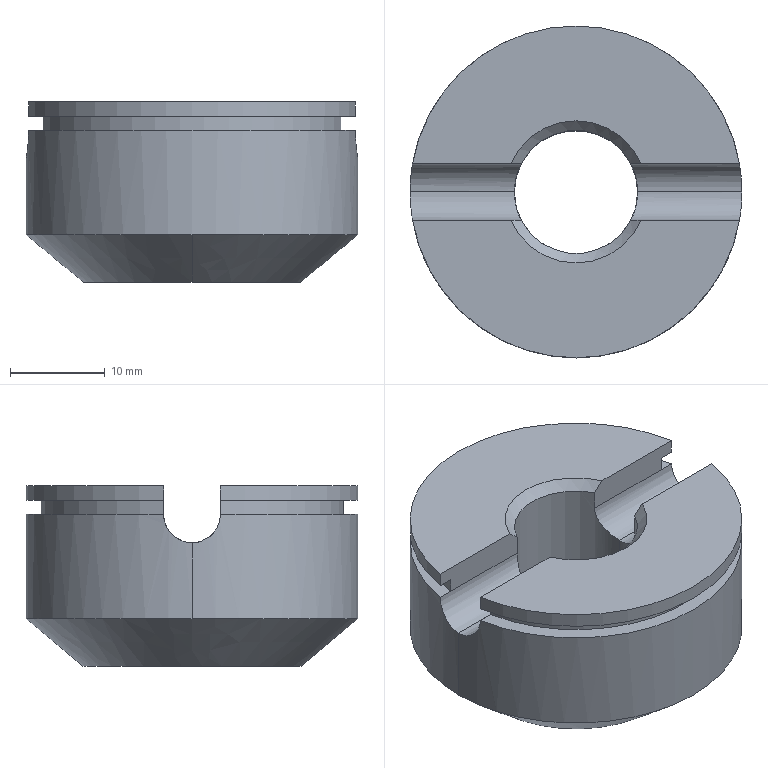Part | SolidWorks | features ICE 4, Blend 1, Chamfer 1, Extrusion 1 | 1 solid | 27 faces | box 35 x 35 x 19 mm | volume 13347 mm3 | cylinder 12 | plane 11 | spline 2 | cone 2 | commonest cylinder face diameters 6 x4 35 x4 13 x2 32 x2
STEP:
#1=CARTESIAN_POINT('',(0.,-17.5,0.));
#2=VERTEX_POINT('',#1);
#3=CARTESIAN_POINT('',(17.5,0.,0.));
#4=VERTEX_POINT('',#3);
#5=CARTESIAN_POINT('',(0.,0.,0.));
#6=DIRECTION('',(0.,0.,1.));
#7=DIRECTION('',(1.,0.,0.));
#8=AXIS2_PLACEMENT_3D('',#5,#6,#7);
#9=CIRCLE('',#8,17.5);
#10=EDGE_CURVE('',#2,#4,#9,.T.);
#11=ORIENTED_EDGE('',*,*,#10,.F.);
#12=CARTESIAN_POINT('',(0.,-11.5,-5.));
#13=VERTEX_POINT('',#12);
#14=CARTESIAN_POINT('',(0.,-17.5,0.));
#15=CARTESIAN_POINT('',(0.,-15.5,-1.667));
#16=CARTESIAN_POINT('',(0.,-13.5,-3.333));
#17=CARTESIAN_POINT('',(0.,-11.5,-5.));
#18=B_SPLINE_CURVE_WITH_KNOTS('',3,(#14,#15,#16,#17),.UNSPECIFIED.,.F.,.F.,(4,4),(0.,1.),.UNSPECIFIED.);
#19=EDGE_CURVE('',#2,#13,#18,.T.);
#20=ORIENTED_EDGE('',*,*,#19,.T.);
#21=CARTESIAN_POINT('',(0.,11.5,-5.));
#22=VERTEX_POINT('',#21);
#23=CARTESIAN_POINT('',(0.,0.,-5.));
#24=DIRECTION('',(0.,0.,-1.));
#25=DIRECTION('',(-1.,0.,0.));
#26=AXIS2_PLACEMENT_3D('',#23,#24,#25);
#27=CIRCLE('',#26,11.5);
#28=EDGE_CURVE('',#22,#13,#27,.T.);
#29=ORIENTED_EDGE('',*,*,#28,.F.);
#30=CARTESIAN_POINT('',(0.,17.5,0.));
#31=VERTEX_POINT('',#30);
#32=CARTESIAN_POINT('',(0.,17.5,0.));
#33=CARTESIAN_POINT('',(0.,15.5,-1.667));
#34=CARTESIAN_POINT('',(0.,13.5,-3.333));
#35=CARTESIAN_POINT('',(0.,11.5,-5.));
#36=B_SPLINE_CURVE_WITH_KNOTS('',3,(#32,#33,#34,#35),.UNSPECIFIED.,.F.,.F.,(4,4),(0.,1.),.UNSPECIFIED.);
#37=EDGE_CURVE('',#31,#22,#36,.T.);
#38=ORIENTED_EDGE('',*,*,#37,.F.);
#39=CARTESIAN_POINT('',(0.,0.,0.));
#40=DIRECTION('',(0.,0.,1.));
#41=DIRECTION('',(1.,0.,0.));
#42=AXIS2_PLACEMENT_3D('',#39,#40,#41);
#43=CIRCLE('',#42,17.5);
#44=EDGE_CURVE('',#4,#31,#43,.T.);
#45=ORIENTED_EDGE('',*,*,#44,.F.);
#46=EDGE_LOOP('',(#11,#20,#29,#38,#45));
#47=FACE_OUTER_BOUND('',#46,.T.);
#48=CARTESIAN_POINT('',(0.,17.5,0.));
#49=CARTESIAN_POINT('',(0.,15.5,-1.667));
#50=CARTESIAN_POINT('',(0.,13.5,-3.333));
#51=CARTESIAN_POINT('',(0.,11.5,-5.));
#52=CARTESIAN_POINT('',(0.4829,17.5,0.));
#53=CARTESIAN_POINT('',(0.4277,15.5,-1.667));
#54=CARTESIAN_POINT('',(0.3725,13.5,-3.333));
#55=CARTESIAN_POINT('',(0.3174,11.5,-5.));
#56=CARTESIAN_POINT('',(1.44,17.461,0.));
#57=CARTESIAN_POINT('',(1.275,15.465,-1.667));
#58=CARTESIAN_POINT('',(1.111,13.47,-3.333));
#59=CARTESIAN_POINT('',(0.9461,11.474,-5.));
#60=CARTESIAN_POINT('',(2.843,17.289,0.));
#61=CARTESIAN_POINT('',(2.518,15.313,-1.667));
#62=CARTESIAN_POINT('',(2.193,13.337,-3.333));
#63=CARTESIAN_POINT('',(1.868,11.361,-5.));
#64=CARTESIAN_POINT('',(4.21,17.008,0.));
#65=CARTESIAN_POINT('',(3.729,15.065,-1.667));
#66=CARTESIAN_POINT('',(3.248,13.121,-3.333));
#67=CARTESIAN_POINT('',(2.767,11.177,-5.));
#68=CARTESIAN_POINT('',(12.168,14.701,0.));
#69=CARTESIAN_POINT('',(10.777,13.021,-1.667));
#70=CARTESIAN_POINT('',(9.387,11.341,-3.333));
#71=CARTESIAN_POINT('',(7.996,9.661,-5.));
#72=CARTESIAN_POINT('',(17.5,7.727,0.));
#73=CARTESIAN_POINT('',(15.5,6.844,-1.667));
#74=CARTESIAN_POINT('',(13.5,5.961,-3.333));
#75=CARTESIAN_POINT('',(11.5,5.078,-5.));
#76=CARTESIAN_POINT('',(17.5,-9.659,0.));
#77=CARTESIAN_POINT('',(15.5,-8.555,-1.667));
#78=CARTESIAN_POINT('',(13.5,-7.451,-3.333));
#79=CARTESIAN_POINT('',(11.5,-6.347,-5.));
#80=CARTESIAN_POINT('',(9.659,-17.5,0.));
#81=CARTESIAN_POINT('',(8.555,-15.5,-1.667));
#82=CARTESIAN_POINT('',(7.451,-13.5,-3.333));
#83=CARTESIAN_POINT('',(6.347,-11.5,-5.));
#84=CARTESIAN_POINT('',(-9.659,-17.5,0.));
#85=CARTESIAN_POINT('',(-8.555,-15.5,-1.667));
#86=CARTESIAN_POINT('',(-7.451,-13.5,-3.333));
#87=CARTESIAN_POINT('',(-6.347,-11.5,-5.));
#88=CARTESIAN_POINT('',(-17.5,-9.659,0.));
#89=CARTESIAN_POINT('',(-15.5,-8.555,-1.667));
#90=CARTESIAN_POINT('',(-13.5,-7.451,-3.333));
#91=CARTESIAN_POINT('',(-11.5,-6.347,-5.));
#92=CARTESIAN_POINT('',(-17.5,7.727,0.));
#93=CARTESIAN_POINT('',(-15.5,6.844,-1.667));
#94=CARTESIAN_POINT('',(-13.5,5.961,-3.333));
#95=CARTESIAN_POINT('',(-11.5,5.078,-5.));
#96=CARTESIAN_POINT('',(-12.168,14.701,0.));
#97=CARTESIAN_POINT('',(-10.777,13.021,-1.667));
#98=CARTESIAN_POINT('',(-9.387,11.341,-3.333));
#99=CARTESIAN_POINT('',(-7.996,9.661,-5.));
#100=CARTESIAN_POINT('',(-4.21,17.008,0.));
#101=CARTESIAN_POINT('',(-3.729,15.065,-1.667));
#102=CARTESIAN_POINT('',(-3.248,13.121,-3.333));
#103=CARTESIAN_POINT('',(-2.767,11.177,-5.));
#104=CARTESIAN_POINT('',(-2.843,17.289,0.));
#105=CARTESIAN_POINT('',(-2.518,15.313,-1.667));
#106=CARTESIAN_POINT('',(-2.193,13.337,-3.333));
#107=CARTESIAN_POINT('',(-1.868,11.361,-5.));
#108=CARTESIAN_POINT('',(-1.44,17.461,0.));
#109=CARTESIAN_POINT('',(-1.275,15.465,-1.667));
#110=CARTESIAN_POINT('',(-1.111,13.47,-3.333));
#111=CARTESIAN_POINT('',(-0.9461,11.474,-5.));
#112=CARTESIAN_POINT('',(-0.4829,17.5,0.));
#113=CARTESIAN_POINT('',(-0.4277,15.5,-1.667));
#114=CARTESIAN_POINT('',(-0.3725,13.5,-3.333));
#115=CARTESIAN_POINT('',(-0.3174,11.5,-5.));
#116=CARTESIAN_POINT('',(0.,17.5,0.));
#117=CARTESIAN_POINT('',(0.,15.5,-1.667));
#118=CARTESIAN_POINT('',(0.,13.5,-3.333));
#119=CARTESIAN_POINT('',(0.,11.5,-5.));
#120=B_SPLINE_SURFACE_WITH_KNOTS('',3,3,((#48,#49,#50,#51),(#52,#53,#54,#55),(#56,#57,#58,#59),(#60,#61,#62,#63),(#64,#65,#66,#67),(#68,#69,#70,#71),(#72,#73,#74,#75),(#76,#77,#78,#79),(#80,#81,#82,#83),(#84,#85,#86,#87),(#88,#89,#90,#91),(#92,#93,#94,#95),(#96,#97,#98,#99),(#100,#101,#102,#103),(#104,#105,#106,#107),(#108,#109,#110,#111),(#112,#113,#114,#115),(#116,#117,#118,#119)),.UNSPECIFIED.,.T.,.F.,.F.,(4,1,1,1,1,2,2,2,1,1,1,1,4),(4,4),(0.,0.0125,0.025,0.0375,0.05,0.25,0.5,0.75,0.95,0.9625,0.975,0.9875,1.),(0.,1.),.UNSPECIFIED.);
#121=ADVANCED_FACE('',(#47),#120,.T.);
#122=CARTESIAN_POINT('',(-17.5,0.,8.));
#123=VERTEX_POINT('',#122);
#124=CARTESIAN_POINT('',(-17.241,3.,11.));
#125=VERTEX_POINT('',#124);
#126=CARTESIAN_POINT('',(-17.5,0.,8.));
#127=CARTESIAN_POINT('',(-17.5,0.1959,8.));
#128=CARTESIAN_POINT('',(-17.497,0.395,8.02));
#129=CARTESIAN_POINT('',(-17.484,0.7797,8.096));
#130=CARTESIAN_POINT('',(-17.474,0.9668,8.153));
#131=CARTESIAN_POINT('',(-17.45,1.33,8.304));
#132=CARTESIAN_POINT('',(-17.436,1.505,8.398));
#133=CARTESIAN_POINT('',(-17.405,1.83,8.614));
#134=CARTESIAN_POINT('',(-17.388,1.981,8.739));
#135=CARTESIAN_POINT('',(-17.354,2.261,9.018));
#136=CARTESIAN_POINT('',(-17.337,2.384,9.169));
#137=CARTESIAN_POINT('',(-17.306,2.601,9.493));
#138=CARTESIAN_POINT('',(-17.291,2.695,9.669));
#139=CARTESIAN_POINT('',(-17.267,2.846,10.031));
#140=CARTESIAN_POINT('',(-17.258,2.903,10.218));
#141=CARTESIAN_POINT('',(-17.244,2.98,10.603));
#142=CARTESIAN_POINT('',(-17.241,3.,10.802));
#143=CARTESIAN_POINT('',(-17.241,3.,11.));
#144=B_SPLINE_CURVE_WITH_KNOTS('',3,(#126,#127,#128,#129,#130,#131,#132,#133,#134,#135,#136,#137,#138,#139,#140,#141,#142,#143),.UNSPECIFIED.,.F.,.F.,(4,2,2,2,2,2,2,2,4),(0.004699,0.005286,0.005873,0.00646,0.007047,0.007634,0.008221,0.008807,0.009394),.UNSPECIFIED.);
#145=EDGE_CURVE('',#123,#125,#144,.T.);
#146=ORIENTED_EDGE('',*,*,#145,.F.);
#147=CARTESIAN_POINT('',(-6.5,0.,8.));
#148=VERTEX_POINT('',#147);
#149=CARTESIAN_POINT('',(-24.5,0.,8.));
#150=DIRECTION('',(1.,0.,0.));
#151=VECTOR('',#150,1000.);
#152=LINE('',#149,#151);
#153=EDGE_CURVE('',#123,#148,#152,.T.);
#154=ORIENTED_EDGE('',*,*,#153,.T.);
#155=CARTESIAN_POINT('',(-5.766,3.,11.));
#156=VERTEX_POINT('',#155);
#157=CARTESIAN_POINT('',(-5.766,3.,11.));
#158=CARTESIAN_POINT('',(-5.766,3.,10.799));
#159=CARTESIAN_POINT('',(-5.777,2.98,10.601));
#160=CARTESIAN_POINT('',(-5.816,2.902,10.214));
#161=CARTESIAN_POINT('',(-5.846,2.843,10.022));
#162=CARTESIAN_POINT('',(-5.917,2.691,9.66));
#163=CARTESIAN_POINT('',(-5.959,2.599,9.489));
#164=CARTESIAN_POINT('',(-6.049,2.382,9.165));
#165=CARTESIAN_POINT('',(-6.097,2.257,9.015));
#166=CARTESIAN_POINT('',(-6.191,1.985,8.742));
#167=CARTESIAN_POINT('',(-6.238,1.834,8.618));
#168=CARTESIAN_POINT('',(-6.325,1.509,8.4));
#169=CARTESIAN_POINT('',(-6.363,1.338,8.308));
#170=CARTESIAN_POINT('',(-6.429,0.9774,8.157));
#171=CARTESIAN_POINT('',(-6.455,0.7852,8.098));
#172=CARTESIAN_POINT('',(-6.491,0.3961,8.02));
#173=CARTESIAN_POINT('',(-6.5,0.1993,8.));
#174=CARTESIAN_POINT('',(-6.5,0.,8.));
#175=B_SPLINE_CURVE_WITH_KNOTS('',3,(#157,#158,#159,#160,#161,#162,#163,#164,#165,#166,#167,#168,#169,#170,#171,#172,#173,#174),.UNSPECIFIED.,.F.,.F.,(4,2,2,2,2,2,2,2,4),(0.,0.0005949,0.00119,0.001785,0.00238,0.002975,0.00357,0.004165,0.004759),.UNSPECIFIED.);
#176=EDGE_CURVE('',#156,#148,#175,.T.);
#177=ORIENTED_EDGE('',*,*,#176,.F.);
#178=CARTESIAN_POINT('',(-15.716,3.,11.));
#179=VERTEX_POINT('',#178);
#180=CARTESIAN_POINT('',(-24.5,3.,11.));
#181=DIRECTION('',(1.,0.,0.));
#182=VECTOR('',#181,1000.);
#183=LINE('',#180,#182);
#184=EDGE_CURVE('',#179,#156,#183,.T.);
#185=ORIENTED_EDGE('',*,*,#184,.F.);
#186=CARTESIAN_POINT('',(-24.5,3.,11.));
#187=DIRECTION('',(1.,0.,0.));
#188=VECTOR('',#187,1000.);
#189=LINE('',#186,#188);
#190=EDGE_CURVE('',#125,#179,#189,.T.);
#191=ORIENTED_EDGE('',*,*,#190,.F.);
#192=EDGE_LOOP('',(#146,#154,#177,#185,#191));
#193=FACE_OUTER_BOUND('',#192,.T.);
#194=CARTESIAN_POINT('',(-24.5,0.,11.));
#195=DIRECTION('',(1.,0.,0.));
#196=DIRECTION('',(0.,0.,-1.));
#197=AXIS2_PLACEMENT_3D('',#194,#195,#196);
#198=CYLINDRICAL_SURFACE('',#197,3.);
#199=ADVANCED_FACE('',(#193),#198,.F.);
#200=CARTESIAN_POINT('',(6.5,0.,8.));
#201=VERTEX_POINT('',#200);
#202=CARTESIAN_POINT('',(5.766,3.,11.));
#203=VERTEX_POINT('',#202);
#204=CARTESIAN_POINT('',(6.5,0.,8.));
#205=CARTESIAN_POINT('',(6.5,0.1989,8.));
#206=CARTESIAN_POINT('',(6.491,0.4002,8.02));
#207=CARTESIAN_POINT('',(6.455,0.7874,8.098));
#208=CARTESIAN_POINT('',(6.429,0.9772,8.157));
#209=CARTESIAN_POINT('',(6.363,1.342,8.309));
#210=CARTESIAN_POINT('',(6.324,1.513,8.402));
#211=CARTESIAN_POINT('',(6.238,1.835,8.619));
#212=CARTESIAN_POINT('',(6.191,1.987,8.744));
#213=CARTESIAN_POINT('',(6.096,2.259,9.017));
#214=CARTESIAN_POINT('',(6.049,2.382,9.166));
#215=CARTESIAN_POINT('',(5.959,2.599,9.489));
#216=CARTESIAN_POINT('',(5.917,2.692,9.662));
#217=CARTESIAN_POINT('',(5.811,2.917,10.2));
#218=CARTESIAN_POINT('',(5.766,3.,10.598));
#219=CARTESIAN_POINT('',(5.766,3.,11.));
#220=B_SPLINE_CURVE_WITH_KNOTS('',3,(#204,#205,#206,#207,#208,#209,#210,#211,#212,#213,#214,#215,#216,#217,#218,#219),.UNSPECIFIED.,.F.,.F.,(4,2,2,2,2,2,2,4),(0.004759,0.005353,0.005947,0.006541,0.007135,0.007729,0.008323,0.00951),.UNSPECIFIED.);
#221=EDGE_CURVE('',#201,#203,#220,.T.);
#222=ORIENTED_EDGE('',*,*,#221,.F.);
#223=CARTESIAN_POINT('',(17.5,0.,8.));
#224=VERTEX_POINT('',#223);
#225=CARTESIAN_POINT('',(-24.5,0.,8.));
#226=DIRECTION('',(1.,0.,0.));
#227=VECTOR('',#226,1000.);
#228=LINE('',#225,#227);
#229=EDGE_CURVE('',#201,#224,#228,.T.);
#230=ORIENTED_EDGE('',*,*,#229,.T.);
#231=CARTESIAN_POINT('',(17.241,3.,11.));
#232=VERTEX_POINT('',#231);
#233=CARTESIAN_POINT('',(17.241,3.,11.));
#234=CARTESIAN_POINT('',(17.241,3.,10.801));
#235=CARTESIAN_POINT('',(17.244,2.98,10.606));
#236=CARTESIAN_POINT('',(17.257,2.904,10.222));
#237=CARTESIAN_POINT('',(17.267,2.846,10.031));
#238=CARTESIAN_POINT('',(17.291,2.695,9.668));
#239=CARTESIAN_POINT('',(17.306,2.603,9.496));
#240=CARTESIAN_POINT('',(17.337,2.385,9.17));
#241=CARTESIAN_POINT('',(17.354,2.259,9.016));
#242=CARTESIAN_POINT('',(17.388,1.982,8.74));
#243=CARTESIAN_POINT('',(17.405,1.831,8.616));
#244=CARTESIAN_POINT('',(17.436,1.503,8.396));
#245=CARTESIAN_POINT('',(17.45,1.329,8.303));
#246=CARTESIAN_POINT('',(17.474,0.9682,8.154));
#247=CARTESIAN_POINT('',(17.484,0.7787,8.096));
#248=CARTESIAN_POINT('',(17.497,0.3911,8.019));
#249=CARTESIAN_POINT('',(17.5,0.1961,8.));
#250=CARTESIAN_POINT('',(17.5,0.,8.));
#251=B_SPLINE_CURVE_WITH_KNOTS('',3,(#233,#234,#235,#236,#237,#238,#239,#240,#241,#242,#243,#244,#245,#246,#247,#248,#249,#250),.UNSPECIFIED.,.F.,.F.,(4,2,2,2,2,2,2,2,4),(0.,0.0005874,0.001175,0.001762,0.00235,0.002937,0.003525,0.004112,0.004699),.UNSPECIFIED.);
#252=EDGE_CURVE('',#232,#224,#251,.T.);
#253=ORIENTED_EDGE('',*,*,#252,.F.);
#254=CARTESIAN_POINT('',(15.716,3.,11.));
#255=VERTEX_POINT('',#254);
#256=CARTESIAN_POINT('',(-24.5,3.,11.));
#257=DIRECTION('',(1.,0.,0.));
#258=VECTOR('',#257,1000.);
#259=LINE('',#256,#258);
#260=EDGE_CURVE('',#255,#232,#259,.T.);
#261=ORIENTED_EDGE('',*,*,#260,.F.);
#262=CARTESIAN_POINT('',(-24.5,3.,11.));
#263=DIRECTION('',(1.,0.,0.));
#264=VECTOR('',#263,1000.);
#265=LINE('',#262,#264);
#266=EDGE_CURVE('',#203,#255,#265,.T.);
#267=ORIENTED_EDGE('',*,*,#266,.F.);
#268=EDGE_LOOP('',(#222,#230,#253,#261,#267));
#269=FACE_OUTER_BOUND('',#268,.T.);
#270=CARTESIAN_POINT('',(-24.5,0.,11.));
#271=DIRECTION('',(1.,0.,0.));
#272=DIRECTION('',(0.,0.,-1.));
#273=AXIS2_PLACEMENT_3D('',#270,#271,#272);
#274=CYLINDRICAL_SURFACE('',#273,3.);
#275=ADVANCED_FACE('',(#269),#274,.F.);
#276=CARTESIAN_POINT('',(6.5,0.,-5.));
#277=VERTEX_POINT('',#276);
#278=CARTESIAN_POINT('',(-6.5,0.,-5.));
#279=VERTEX_POINT('',#278);
#280=CARTESIAN_POINT('',(0.,0.,-5.));
#281=DIRECTION('',(0.,0.,-1.));
#282=DIRECTION('',(-1.,0.,0.));
#283=AXIS2_PLACEMENT_3D('',#280,#281,#282);
#284=CIRCLE('',#283,6.5);
#285=EDGE_CURVE('',#277,#279,#284,.T.);
#286=ORIENTED_EDGE('',*,*,#285,.T.);
#287=CARTESIAN_POINT('',(-6.5,0.,-5.));
#288=DIRECTION('',(0.,0.,1.));
#289=VECTOR('',#288,1000.);
#290=LINE('',#287,#289);
#291=EDGE_CURVE('',#279,#148,#290,.T.);
#292=ORIENTED_EDGE('',*,*,#291,.T.);
#293=CARTESIAN_POINT('',(-5.766,-3.,11.));
#294=VERTEX_POINT('',#293);
#295=CARTESIAN_POINT('',(-6.5,0.,8.));
#296=CARTESIAN_POINT('',(-6.5,-0.1989,8.));
#297=CARTESIAN_POINT('',(-6.491,-0.4002,8.02));
#298=CARTESIAN_POINT('',(-6.455,-0.7874,8.098));
#299=CARTESIAN_POINT('',(-6.429,-0.9772,8.157));
#300=CARTESIAN_POINT('',(-6.363,-1.342,8.309));
#301=CARTESIAN_POINT('',(-6.324,-1.513,8.402));
#302=CARTESIAN_POINT('',(-6.238,-1.835,8.619));
#303=CARTESIAN_POINT('',(-6.191,-1.987,8.744));
#304=CARTESIAN_POINT('',(-6.096,-2.259,9.017));
#305=CARTESIAN_POINT('',(-6.049,-2.382,9.166));
#306=CARTESIAN_POINT('',(-5.959,-2.599,9.489));
#307=CARTESIAN_POINT('',(-5.917,-2.692,9.662));
#308=CARTESIAN_POINT('',(-5.811,-2.917,10.2));
#309=CARTESIAN_POINT('',(-5.766,-3.,10.598));
#310=CARTESIAN_POINT('',(-5.766,-3.,11.));
#311=B_SPLINE_CURVE_WITH_KNOTS('',3,(#295,#296,#297,#298,#299,#300,#301,#302,#303,#304,#305,#306,#307,#308,#309,#310),.UNSPECIFIED.,.F.,.F.,(4,2,2,2,2,2,2,4),(0.004759,0.005353,0.005947,0.006541,0.007135,0.007729,0.008323,0.00951),.UNSPECIFIED.);
#312=EDGE_CURVE('',#148,#294,#311,.T.);
#313=ORIENTED_EDGE('',*,*,#312,.T.);
#314=CARTESIAN_POINT('',(-5.766,-3.,13.));
#315=VERTEX_POINT('',#314);
#316=CARTESIAN_POINT('',(-5.766,-3.,-5.));
#317=DIRECTION('',(0.,0.,1.));
#318=VECTOR('',#317,1000.);
#319=LINE('',#316,#318);
#320=EDGE_CURVE('',#294,#315,#319,.T.);
#321=ORIENTED_EDGE('',*,*,#320,.T.);
#322=CARTESIAN_POINT('',(5.766,-3.,13.));
#323=VERTEX_POINT('',#322);
#324=CARTESIAN_POINT('',(0.,0.,13.));
#325=DIRECTION('',(0.,0.,1.));
#326=DIRECTION('',(1.,0.,0.));
#327=AXIS2_PLACEMENT_3D('',#324,#325,#326);
#328=CIRCLE('',#327,6.5);
#329=EDGE_CURVE('',#315,#323,#328,.T.);
#330=ORIENTED_EDGE('',*,*,#329,.T.);
#331=CARTESIAN_POINT('',(5.766,-3.,11.));
#332=VERTEX_POINT('',#331);
#333=CARTESIAN_POINT('',(5.766,-3.,-5.));
#334=DIRECTION('',(0.,0.,-1.));
#335=VECTOR('',#334,1000.);
#336=LINE('',#333,#335);
#337=EDGE_CURVE('',#323,#332,#336,.T.);
#338=ORIENTED_EDGE('',*,*,#337,.T.);
#339=CARTESIAN_POINT('',(5.766,-3.,11.));
#340=CARTESIAN_POINT('',(5.766,-3.,10.799));
#341=CARTESIAN_POINT('',(5.777,-2.98,10.601));
#342=CARTESIAN_POINT('',(5.816,-2.902,10.214));
#343=CARTESIAN_POINT('',(5.846,-2.843,10.022));
#344=CARTESIAN_POINT('',(5.917,-2.691,9.66));
#345=CARTESIAN_POINT('',(5.959,-2.599,9.489));
#346=CARTESIAN_POINT('',(6.049,-2.382,9.165));
#347=CARTESIAN_POINT('',(6.097,-2.257,9.015));
#348=CARTESIAN_POINT('',(6.191,-1.985,8.742));
#349=CARTESIAN_POINT('',(6.238,-1.834,8.618));
#350=CARTESIAN_POINT('',(6.325,-1.509,8.4));
#351=CARTESIAN_POINT('',(6.363,-1.338,8.308));
#352=CARTESIAN_POINT('',(6.429,-0.9774,8.157));
#353=CARTESIAN_POINT('',(6.455,-0.7852,8.098));
#354=CARTESIAN_POINT('',(6.491,-0.3961,8.02));
#355=CARTESIAN_POINT('',(6.5,-0.1993,8.));
#356=CARTESIAN_POINT('',(6.5,0.,8.));
#357=B_SPLINE_CURVE_WITH_KNOTS('',3,(#339,#340,#341,#342,#343,#344,#345,#346,#347,#348,#349,#350,#351,#352,#353,#354,#355,#356),.UNSPECIFIED.,.F.,.F.,(4,2,2,2,2,2,2,2,4),(0.,0.0005949,0.00119,0.001785,0.00238,0.002975,0.00357,0.004165,0.004759),.UNSPECIFIED.);
#358=EDGE_CURVE('',#332,#201,#357,.T.);
#359=ORIENTED_EDGE('',*,*,#358,.T.);
#360=CARTESIAN_POINT('',(6.5,0.,-5.));
#361=DIRECTION('',(0.,0.,1.));
#362=VECTOR('',#361,1000.);
#363=LINE('',#360,#362);
#364=EDGE_CURVE('',#277,#201,#363,.T.);
#365=ORIENTED_EDGE('',*,*,#364,.F.);
#366=EDGE_LOOP('',(#286,#292,#313,#321,#330,#338,#359,#365));
#367=FACE_OUTER_BOUND('',#366,.T.);
#368=CARTESIAN_POINT('',(0.,0.,-5.));
#369=DIRECTION('',(0.,0.,1.));
#370=DIRECTION('',(1.,0.,0.));
#371=AXIS2_PLACEMENT_3D('',#368,#369,#370);
#372=CYLINDRICAL_SURFACE('',#371,6.5);
#373=ADVANCED_FACE('',(#367),#372,.F.);
#374=ORIENTED_EDGE('',*,*,#252,.T.);
#375=CARTESIAN_POINT('',(17.5,0.,14.));
#376=DIRECTION('',(0.,0.,-1.));
#377=VECTOR('',#376,1000.);
#378=LINE('',#375,#377);
#379=EDGE_CURVE('',#224,#4,#378,.T.);
#380=ORIENTED_EDGE('',*,*,#379,.T.);
#381=ORIENTED_EDGE('',*,*,#44,.T.);
#382=CARTESIAN_POINT('',(-17.5,0.,0.));
#383=VERTEX_POINT('',#382);
#384=CARTESIAN_POINT('',(0.,0.,0.));
#385=DIRECTION('',(0.,0.,1.));
#386=DIRECTION('',(1.,0.,0.));
#387=AXIS2_PLACEMENT_3D('',#384,#385,#386);
#388=CIRCLE('',#387,17.5);
#389=EDGE_CURVE('',#31,#383,#388,.T.);
#390=ORIENTED_EDGE('',*,*,#389,.T.);
#391=CARTESIAN_POINT('',(-17.5,0.,14.));
#392=DIRECTION('',(0.,0.,-1.));
#393=VECTOR('',#392,1000.);
#394=LINE('',#391,#393);
#395=EDGE_CURVE('',#123,#383,#394,.T.);
#396=ORIENTED_EDGE('',*,*,#395,.F.);
#397=ORIENTED_EDGE('',*,*,#145,.T.);
#398=CARTESIAN_POINT('',(0.,0.,11.));
#399=DIRECTION('',(0.,0.,1.));
#400=DIRECTION('',(1.,0.,0.));
#401=AXIS2_PLACEMENT_3D('',#398,#399,#400);
#402=CIRCLE('',#401,17.5);
#403=EDGE_CURVE('',#232,#125,#402,.T.);
#404=ORIENTED_EDGE('',*,*,#403,.F.);
#405=EDGE_LOOP('',(#374,#380,#381,#390,#396,#397,#404));
#406=FACE_OUTER_BOUND('',#405,.T.);
#407=CARTESIAN_POINT('',(0.,0.,14.));
#408=DIRECTION('',(0.,0.,-1.));
#409=DIRECTION('',(-1.,0.,0.));
#410=AXIS2_PLACEMENT_3D('',#407,#408,#409);
#411=CYLINDRICAL_SURFACE('',#410,17.5);
#412=ADVANCED_FACE('',(#406),#411,.T.);
#413=ORIENTED_EDGE('',*,*,#379,.F.);
#414=CARTESIAN_POINT('',(17.241,-3.,11.));
#415=VERTEX_POINT('',#414);
#416=CARTESIAN_POINT('',(17.5,0.,8.));
#417=CARTESIAN_POINT('',(17.5,-0.1959,8.));
#418=CARTESIAN_POINT('',(17.497,-0.395,8.02));
#419=CARTESIAN_POINT('',(17.484,-0.7797,8.096));
#420=CARTESIAN_POINT('',(17.474,-0.9668,8.153));
#421=CARTESIAN_POINT('',(17.45,-1.33,8.304));
#422=CARTESIAN_POINT('',(17.436,-1.505,8.398));
#423=CARTESIAN_POINT('',(17.405,-1.83,8.614));
#424=CARTESIAN_POINT('',(17.388,-1.981,8.739));
#425=CARTESIAN_POINT('',(17.354,-2.261,9.018));
#426=CARTESIAN_POINT('',(17.337,-2.384,9.169));
#427=CARTESIAN_POINT('',(17.306,-2.601,9.493));
#428=CARTESIAN_POINT('',(17.291,-2.695,9.669));
#429=CARTESIAN_POINT('',(17.267,-2.846,10.031));
#430=CARTESIAN_POINT('',(17.258,-2.903,10.218));
#431=CARTESIAN_POINT('',(17.244,-2.98,10.603));
#432=CARTESIAN_POINT('',(17.241,-3.,10.802));
#433=CARTESIAN_POINT('',(17.241,-3.,11.));
#434=B_SPLINE_CURVE_WITH_KNOTS('',3,(#416,#417,#418,#419,#420,#421,#422,#423,#424,#425,#426,#427,#428,#429,#430,#431,#432,#433),.UNSPECIFIED.,.F.,.F.,(4,2,2,2,2,2,2,2,4),(0.004699,0.005286,0.005873,0.00646,0.007047,0.007634,0.008221,0.008807,0.009394),.UNSPECIFIED.);
#435=EDGE_CURVE('',#224,#415,#434,.T.);
#436=ORIENTED_EDGE('',*,*,#435,.T.);
#437=CARTESIAN_POINT('',(-17.241,-3.,11.));
#438=VERTEX_POINT('',#437);
#439=CARTESIAN_POINT('',(0.,0.,11.));
#440=DIRECTION('',(0.,0.,1.));
#441=DIRECTION('',(1.,0.,0.));
#442=AXIS2_PLACEMENT_3D('',#439,#440,#441);
#443=CIRCLE('',#442,17.5);
#444=EDGE_CURVE('',#438,#415,#443,.T.);
#445=ORIENTED_EDGE('',*,*,#444,.F.);
#446=CARTESIAN_POINT('',(-17.241,-3.,11.));
#447=CARTESIAN_POINT('',(-17.241,-3.,10.801));
#448=CARTESIAN_POINT('',(-17.244,-2.98,10.606));
#449=CARTESIAN_POINT('',(-17.257,-2.904,10.222));
#450=CARTESIAN_POINT('',(-17.267,-2.846,10.031));
#451=CARTESIAN_POINT('',(-17.291,-2.695,9.668));
#452=CARTESIAN_POINT('',(-17.306,-2.603,9.496));
#453=CARTESIAN_POINT('',(-17.337,-2.385,9.17));
#454=CARTESIAN_POINT('',(-17.354,-2.259,9.016));
#455=CARTESIAN_POINT('',(-17.388,-1.982,8.74));
#456=CARTESIAN_POINT('',(-17.405,-1.831,8.616));
#457=CARTESIAN_POINT('',(-17.436,-1.503,8.396));
#458=CARTESIAN_POINT('',(-17.45,-1.329,8.303));
#459=CARTESIAN_POINT('',(-17.474,-0.9682,8.154));
#460=CARTESIAN_POINT('',(-17.484,-0.7787,8.096));
#461=CARTESIAN_POINT('',(-17.497,-0.3911,8.019));
#462=CARTESIAN_POINT('',(-17.5,-0.1961,8.));
#463=CARTESIAN_POINT('',(-17.5,0.,8.));
#464=B_SPLINE_CURVE_WITH_KNOTS('',3,(#446,#447,#448,#449,#450,#451,#452,#453,#454,#455,#456,#457,#458,#459,#460,#461,#462,#463),.UNSPECIFIED.,.F.,.F.,(4,2,2,2,2,2,2,2,4),(0.,0.0005874,0.001175,0.001762,0.00235,0.002937,0.003525,0.004112,0.004699),.UNSPECIFIED.);
#465=EDGE_CURVE('',#438,#123,#464,.T.);
#466=ORIENTED_EDGE('',*,*,#465,.T.);
#467=ORIENTED_EDGE('',*,*,#395,.T.);
#468=CARTESIAN_POINT('',(0.,0.,0.));
#469=DIRECTION('',(0.,0.,1.));
#470=DIRECTION('',(1.,0.,0.));
#471=AXIS2_PLACEMENT_3D('',#468,#469,#470);
#472=CIRCLE('',#471,17.5);
#473=EDGE_CURVE('',#383,#2,#472,.T.);
#474=ORIENTED_EDGE('',*,*,#473,.T.);
#475=ORIENTED_EDGE('',*,*,#10,.T.);
#476=EDGE_LOOP('',(#413,#436,#445,#466,#467,#474,#475));
#477=FACE_OUTER_BOUND('',#476,.T.);
#478=CARTESIAN_POINT('',(0.,0.,14.));
#479=DIRECTION('',(0.,0.,-1.));
#480=DIRECTION('',(-1.,0.,0.));
#481=AXIS2_PLACEMENT_3D('',#478,#479,#480);
#482=CYLINDRICAL_SURFACE('',#481,17.5);
#483=ADVANCED_FACE('',(#477),#482,.T.);
#484=CARTESIAN_POINT('',(17.241,3.,14.));
#485=VERTEX_POINT('',#484);
#486=CARTESIAN_POINT('',(17.241,3.,12.5));
#487=VERTEX_POINT('',#486);
#488=CARTESIAN_POINT('',(17.241,3.,14.));
#489=DIRECTION('',(0.,0.,-1.));
#490=VECTOR('',#489,1000.);
#491=LINE('',#488,#490);
#492=EDGE_CURVE('',#485,#487,#491,.T.);
#493=ORIENTED_EDGE('',*,*,#492,.T.);
#494=CARTESIAN_POINT('',(-17.241,3.,12.5));
#495=VERTEX_POINT('',#494);
#496=CARTESIAN_POINT('',(0.,0.,12.5));
#497=DIRECTION('',(0.,0.,1.));
#498=DIRECTION('',(1.,0.,0.));
#499=AXIS2_PLACEMENT_3D('',#496,#497,#498);
#500=CIRCLE('',#499,17.5);
#501=EDGE_CURVE('',#487,#495,#500,.T.);
#502=ORIENTED_EDGE('',*,*,#501,.T.);
#503=CARTESIAN_POINT('',(-17.241,3.,14.));
#504=VERTEX_POINT('',#503);
#505=CARTESIAN_POINT('',(-17.241,3.,14.));
#506=DIRECTION('',(0.,0.,1.));
#507=VECTOR('',#506,1000.);
#508=LINE('',#505,#507);
#509=EDGE_CURVE('',#495,#504,#508,.T.);
#510=ORIENTED_EDGE('',*,*,#509,.T.);
#511=CARTESIAN_POINT('',(0.,0.,14.));
#512=DIRECTION('',(0.,0.,1.));
#513=DIRECTION('',(1.,0.,0.));
#514=AXIS2_PLACEMENT_3D('',#511,#512,#513);
#515=CIRCLE('',#514,17.5);
#516=EDGE_CURVE('',#485,#504,#515,.T.);
#517=ORIENTED_EDGE('',*,*,#516,.F.);
#518=EDGE_LOOP('',(#493,#502,#510,#517));
#519=FACE_OUTER_BOUND('',#518,.T.);
#520=CARTESIAN_POINT('',(0.,0.,14.));
#521=DIRECTION('',(0.,0.,-1.));
#522=DIRECTION('',(-1.,0.,0.));
#523=AXIS2_PLACEMENT_3D('',#520,#521,#522);
#524=CYLINDRICAL_SURFACE('',#523,17.5);
#525=ADVANCED_FACE('',(#519),#524,.T.);
#526=CARTESIAN_POINT('',(6.874,-3.,14.));
#527=VERTEX_POINT('',#526);
#528=CARTESIAN_POINT('',(17.241,-3.,14.));
#529=VERTEX_POINT('',#528);
#530=CARTESIAN_POINT('',(-24.5,-3.,14.));
#531=DIRECTION('',(1.,0.,0.));
#532=VECTOR('',#531,1000.);
#533=LINE('',#530,#532);
#534=EDGE_CURVE('',#527,#529,#533,.T.);
#535=ORIENTED_EDGE('',*,*,#534,.F.);
#536=CARTESIAN_POINT('',(-6.874,-3.,14.));
#537=VERTEX_POINT('',#536);
#538=CARTESIAN_POINT('',(0.,0.,14.));
#539=DIRECTION('',(0.,0.,-1.));
#540=DIRECTION('',(1.,0.,0.));
#541=AXIS2_PLACEMENT_3D('',#538,#539,#540);
#542=CIRCLE('',#541,7.5);
#543=EDGE_CURVE('',#527,#537,#542,.T.);
#544=ORIENTED_EDGE('',*,*,#543,.T.);
#545=CARTESIAN_POINT('',(-17.241,-3.,14.));
#546=VERTEX_POINT('',#545);
#547=CARTESIAN_POINT('',(-24.5,-3.,14.));
#548=DIRECTION('',(1.,0.,0.));
#549=VECTOR('',#548,1000.);
#550=LINE('',#547,#549);
#551=EDGE_CURVE('',#546,#537,#550,.T.);
#552=ORIENTED_EDGE('',*,*,#551,.F.);
#553=CARTESIAN_POINT('',(0.,0.,14.));
#554=DIRECTION('',(0.,0.,1.));
#555=DIRECTION('',(1.,0.,0.));
#556=AXIS2_PLACEMENT_3D('',#553,#554,#555);
#557=CIRCLE('',#556,17.5);
#558=EDGE_CURVE('',#546,#529,#557,.T.);
#559=ORIENTED_EDGE('',*,*,#558,.T.);
#560=EDGE_LOOP('',(#535,#544,#552,#559));
#561=FACE_OUTER_BOUND('',#560,.T.);
#562=CARTESIAN_POINT('',(0.,0.,14.));
#563=DIRECTION('',(0.,0.,1.));
#564=DIRECTION('',(1.,0.,0.));
#565=AXIS2_PLACEMENT_3D('',#562,#563,#564);
#566=PLANE('',#565);
#567=ADVANCED_FACE('',(#561),#566,.T.);
#568=CARTESIAN_POINT('',(-17.241,-3.,12.5));
#569=VERTEX_POINT('',#568);
#570=CARTESIAN_POINT('',(-17.241,-3.,14.));
#571=DIRECTION('',(0.,0.,-1.));
#572=VECTOR('',#571,1000.);
#573=LINE('',#570,#572);
#574=EDGE_CURVE('',#546,#569,#573,.T.);
#575=ORIENTED_EDGE('',*,*,#574,.T.);
#576=CARTESIAN_POINT('',(17.241,-3.,12.5));
#577=VERTEX_POINT('',#576);
#578=CARTESIAN_POINT('',(0.,0.,12.5));
#579=DIRECTION('',(0.,0.,1.));
#580=DIRECTION('',(1.,0.,0.));
#581=AXIS2_PLACEMENT_3D('',#578,#579,#580);
#582=CIRCLE('',#581,17.5);
#583=EDGE_CURVE('',#569,#577,#582,.T.);
#584=ORIENTED_EDGE('',*,*,#583,.T.);
#585=CARTESIAN_POINT('',(17.241,-3.,14.));
#586=DIRECTION('',(0.,0.,1.));
#587=VECTOR('',#586,1000.);
#588=LINE('',#585,#587);
#589=EDGE_CURVE('',#577,#529,#588,.T.);
#590=ORIENTED_EDGE('',*,*,#589,.T.);
#591=ORIENTED_EDGE('',*,*,#558,.F.);
#592=EDGE_LOOP('',(#575,#584,#590,#591));
#593=FACE_OUTER_BOUND('',#592,.T.);
#594=CARTESIAN_POINT('',(0.,0.,14.));
#595=DIRECTION('',(0.,0.,-1.));
#596=DIRECTION('',(-1.,0.,0.));
#597=AXIS2_PLACEMENT_3D('',#594,#595,#596);
#598=CYLINDRICAL_SURFACE('',#597,17.5);
#599=ADVANCED_FACE('',(#593),#598,.T.);
#600=CARTESIAN_POINT('',(-6.874,3.,14.));
#601=VERTEX_POINT('',#600);
#602=CARTESIAN_POINT('',(-24.5,3.,14.));
#603=DIRECTION('',(1.,0.,0.));
#604=VECTOR('',#603,1000.);
#605=LINE('',#602,#604);
#606=EDGE_CURVE('',#504,#601,#605,.T.);
#607=ORIENTED_EDGE('',*,*,#606,.T.);
#608=CARTESIAN_POINT('',(6.874,3.,14.));
#609=VERTEX_POINT('',#608);
#610=CARTESIAN_POINT('',(0.,0.,14.));
#611=DIRECTION('',(0.,0.,-1.));
#612=DIRECTION('',(1.,0.,0.));
#613=AXIS2_PLACEMENT_3D('',#610,#611,#612);
#614=CIRCLE('',#613,7.5);
#615=EDGE_CURVE('',#601,#609,#614,.T.);
#616=ORIENTED_EDGE('',*,*,#615,.T.);
#617=CARTESIAN_POINT('',(-24.5,3.,14.));
#618=DIRECTION('',(1.,0.,0.));
#619=VECTOR('',#618,1000.);
#620=LINE('',#617,#619);
#621=EDGE_CURVE('',#609,#485,#620,.T.);
#622=ORIENTED_EDGE('',*,*,#621,.T.);
#623=ORIENTED_EDGE('',*,*,#516,.T.);
#624=EDGE_LOOP('',(#607,#616,#622,#623));
#625=FACE_OUTER_BOUND('',#624,.T.);
#626=CARTESIAN_POINT('',(0.,0.,14.));
#627=DIRECTION('',(0.,0.,1.));
#628=DIRECTION('',(1.,0.,0.));
#629=AXIS2_PLACEMENT_3D('',#626,#627,#628);
#630=PLANE('',#629);
#631=ADVANCED_FACE('',(#625),#630,.T.);
#632=ORIENTED_EDGE('',*,*,#291,.F.);
#633=CARTESIAN_POINT('',(0.,0.,-5.));
#634=DIRECTION('',(0.,0.,-1.));
#635=DIRECTION('',(-1.,0.,0.));
#636=AXIS2_PLACEMENT_3D('',#633,#634,#635);
#637=CIRCLE('',#636,6.5);
#638=EDGE_CURVE('',#279,#277,#637,.T.);
#639=ORIENTED_EDGE('',*,*,#638,.T.);
#640=ORIENTED_EDGE('',*,*,#364,.T.);
#641=ORIENTED_EDGE('',*,*,#221,.T.);
#642=CARTESIAN_POINT('',(5.766,3.,13.));
#643=VERTEX_POINT('',#642);
#644=CARTESIAN_POINT('',(5.766,3.,-5.));
#645=DIRECTION('',(0.,0.,1.));
#646=VECTOR('',#645,1000.);
#647=LINE('',#644,#646);
#648=EDGE_CURVE('',#203,#643,#647,.T.);
#649=ORIENTED_EDGE('',*,*,#648,.T.);
#650=CARTESIAN_POINT('',(-5.766,3.,13.));
#651=VERTEX_POINT('',#650);
#652=CARTESIAN_POINT('',(0.,0.,13.));
#653=DIRECTION('',(0.,0.,1.));
#654=DIRECTION('',(1.,0.,0.));
#655=AXIS2_PLACEMENT_3D('',#652,#653,#654);
#656=CIRCLE('',#655,6.5);
#657=EDGE_CURVE('',#643,#651,#656,.T.);
#658=ORIENTED_EDGE('',*,*,#657,.T.);
#659=CARTESIAN_POINT('',(-5.766,3.,-5.));
#660=DIRECTION('',(0.,0.,-1.));
#661=VECTOR('',#660,1000.);
#662=LINE('',#659,#661);
#663=EDGE_CURVE('',#651,#156,#662,.T.);
#664=ORIENTED_EDGE('',*,*,#663,.T.);
#665=ORIENTED_EDGE('',*,*,#176,.T.);
#666=EDGE_LOOP('',(#632,#639,#640,#641,#649,#658,#664,#665));
#667=FACE_OUTER_BOUND('',#666,.T.);
#668=CARTESIAN_POINT('',(0.,0.,-5.));
#669=DIRECTION('',(0.,0.,1.));
#670=DIRECTION('',(1.,0.,0.));
#671=AXIS2_PLACEMENT_3D('',#668,#669,#670);
#672=CYLINDRICAL_SURFACE('',#671,6.5);
#673=ADVANCED_FACE('',(#667),#672,.F.);
#674=ORIENTED_EDGE('',*,*,#337,.F.);
#675=CARTESIAN_POINT('',(5.766,-3.,13.));
#676=CARTESIAN_POINT('',(6.138,-3.,13.33));
#677=CARTESIAN_POINT('',(6.507,-3.,13.664));
#678=CARTESIAN_POINT('',(6.874,-3.,14.));
#679=B_SPLINE_CURVE_WITH_KNOTS('',3,(#675,#676,#677,#678),.UNSPECIFIED.,.F.,.F.,(4,4),(0.,0.001492),.UNSPECIFIED.);
#680=EDGE_CURVE('',#323,#527,#679,.T.);
#681=ORIENTED_EDGE('',*,*,#680,.T.);
#682=ORIENTED_EDGE('',*,*,#534,.T.);
#683=ORIENTED_EDGE('',*,*,#589,.F.);
#684=CARTESIAN_POINT('',(15.716,-3.,12.5));
#685=VERTEX_POINT('',#684);
#686=CARTESIAN_POINT('',(-24.5,-3.,12.5));
#687=DIRECTION('',(-1.,0.,0.));
#688=VECTOR('',#687,1000.);
#689=LINE('',#686,#688);
#690=EDGE_CURVE('',#577,#685,#689,.T.);
#691=ORIENTED_EDGE('',*,*,#690,.T.);
#692=CARTESIAN_POINT('',(15.716,-3.,11.));
#693=VERTEX_POINT('',#692);
#694=CARTESIAN_POINT('',(15.716,-3.,11.));
#695=DIRECTION('',(0.,0.,1.));
#696=VECTOR('',#695,1000.);
#697=LINE('',#694,#696);
#698=EDGE_CURVE('',#693,#685,#697,.T.);
#699=ORIENTED_EDGE('',*,*,#698,.F.);
#700=CARTESIAN_POINT('',(-24.5,-3.,11.));
#701=DIRECTION('',(1.,0.,0.));
#702=VECTOR('',#701,1000.);
#703=LINE('',#700,#702);
#704=EDGE_CURVE('',#332,#693,#703,.T.);
#705=ORIENTED_EDGE('',*,*,#704,.F.);
#706=EDGE_LOOP('',(#674,#681,#682,#683,#691,#699,#705));
#707=FACE_OUTER_BOUND('',#706,.T.);
#708=CARTESIAN_POINT('',(-24.5,-3.,11.));
#709=DIRECTION('',(0.,-1.,0.));
#710=DIRECTION('',(0.,0.,-1.));
#711=AXIS2_PLACEMENT_3D('',#708,#709,#710);
#712=PLANE('',#711);
#713=ADVANCED_FACE('',(#707),#712,.F.);
#714=ORIENTED_EDGE('',*,*,#621,.F.);
#715=CARTESIAN_POINT('',(6.874,3.,14.));
#716=CARTESIAN_POINT('',(6.507,3.,13.664));
#717=CARTESIAN_POINT('',(6.138,3.,13.33));
#718=CARTESIAN_POINT('',(5.766,3.,13.));
#719=B_SPLINE_CURVE_WITH_KNOTS('',3,(#715,#716,#717,#718),.UNSPECIFIED.,.F.,.F.,(4,4),(0.,0.001492),.UNSPECIFIED.);
#720=EDGE_CURVE('',#609,#643,#719,.T.);
#721=ORIENTED_EDGE('',*,*,#720,.T.);
#722=ORIENTED_EDGE('',*,*,#648,.F.);
#723=ORIENTED_EDGE('',*,*,#266,.T.);
#724=CARTESIAN_POINT('',(15.716,3.,12.5));
#725=VERTEX_POINT('',#724);
#726=CARTESIAN_POINT('',(15.716,3.,11.));
#727=DIRECTION('',(0.,0.,-1.));
#728=VECTOR('',#727,1000.);
#729=LINE('',#726,#728);
#730=EDGE_CURVE('',#725,#255,#729,.T.);
#731=ORIENTED_EDGE('',*,*,#730,.F.);
#732=CARTESIAN_POINT('',(-24.5,3.,12.5));
#733=DIRECTION('',(1.,0.,0.));
#734=VECTOR('',#733,1000.);
#735=LINE('',#732,#734);
#736=EDGE_CURVE('',#725,#487,#735,.T.);
#737=ORIENTED_EDGE('',*,*,#736,.T.);
#738=ORIENTED_EDGE('',*,*,#492,.F.);
#739=EDGE_LOOP('',(#714,#721,#722,#723,#731,#737,#738));
#740=FACE_OUTER_BOUND('',#739,.T.);
#741=CARTESIAN_POINT('',(-24.5,3.,11.));
#742=DIRECTION('',(0.,1.,0.));
#743=DIRECTION('',(0.,0.,1.));
#744=AXIS2_PLACEMENT_3D('',#741,#742,#743);
#745=PLANE('',#744);
#746=ADVANCED_FACE('',(#740),#745,.F.);
#747=ORIENTED_EDGE('',*,*,#229,.F.);
#748=ORIENTED_EDGE('',*,*,#358,.F.);
#749=ORIENTED_EDGE('',*,*,#704,.T.);
#750=CARTESIAN_POINT('',(-24.5,-3.,11.));
#751=DIRECTION('',(-1.,0.,0.));
#752=VECTOR('',#751,1000.);
#753=LINE('',#750,#752);
#754=EDGE_CURVE('',#415,#693,#753,.T.);
#755=ORIENTED_EDGE('',*,*,#754,.F.);
#756=ORIENTED_EDGE('',*,*,#435,.F.);
#757=EDGE_LOOP('',(#747,#748,#749,#755,#756));
#758=FACE_OUTER_BOUND('',#757,.T.);
#759=CARTESIAN_POINT('',(-24.5,0.,11.));
#760=DIRECTION('',(1.,0.,0.));
#761=DIRECTION('',(0.,0.,-1.));
#762=AXIS2_PLACEMENT_3D('',#759,#760,#761);
#763=CYLINDRICAL_SURFACE('',#762,3.);
#764=ADVANCED_FACE('',(#758),#763,.F.);
#765=ORIENTED_EDGE('',*,*,#153,.F.);
#766=ORIENTED_EDGE('',*,*,#465,.F.);
#767=CARTESIAN_POINT('',(-15.716,-3.,11.));
#768=VERTEX_POINT('',#767);
#769=CARTESIAN_POINT('',(-24.5,-3.,11.));
#770=DIRECTION('',(1.,0.,0.));
#771=VECTOR('',#770,1000.);
#772=LINE('',#769,#771);
#773=EDGE_CURVE('',#438,#768,#772,.T.);
#774=ORIENTED_EDGE('',*,*,#773,.T.);
#775=CARTESIAN_POINT('',(-24.5,-3.,11.));
#776=DIRECTION('',(1.,0.,0.));
#777=VECTOR('',#776,1000.);
#778=LINE('',#775,#777);
#779=EDGE_CURVE('',#768,#294,#778,.T.);
#780=ORIENTED_EDGE('',*,*,#779,.T.);
#781=ORIENTED_EDGE('',*,*,#312,.F.);
#782=EDGE_LOOP('',(#765,#766,#774,#780,#781));
#783=FACE_OUTER_BOUND('',#782,.T.);
#784=CARTESIAN_POINT('',(-24.5,0.,11.));
#785=DIRECTION('',(1.,0.,0.));
#786=DIRECTION('',(0.,0.,-1.));
#787=AXIS2_PLACEMENT_3D('',#784,#785,#786);
#788=CYLINDRICAL_SURFACE('',#787,3.);
#789=ADVANCED_FACE('',(#783),#788,.F.);
#790=ORIENTED_EDGE('',*,*,#551,.T.);
#791=CARTESIAN_POINT('',(-6.874,-3.,14.));
#792=CARTESIAN_POINT('',(-6.507,-3.,13.664));
#793=CARTESIAN_POINT('',(-6.138,-3.,13.33));
#794=CARTESIAN_POINT('',(-5.766,-3.,13.));
#795=B_SPLINE_CURVE_WITH_KNOTS('',3,(#791,#792,#793,#794),.UNSPECIFIED.,.F.,.F.,(4,4),(0.,0.001492),.UNSPECIFIED.);
#796=EDGE_CURVE('',#537,#315,#795,.T.);
#797=ORIENTED_EDGE('',*,*,#796,.T.);
#798=ORIENTED_EDGE('',*,*,#320,.F.);
#799=ORIENTED_EDGE('',*,*,#779,.F.);
#800=CARTESIAN_POINT('',(-15.716,-3.,12.5));
#801=VERTEX_POINT('',#800);
#802=CARTESIAN_POINT('',(-15.716,-3.,11.));
#803=DIRECTION('',(0.,0.,-1.));
#804=VECTOR('',#803,1000.);
#805=LINE('',#802,#804);
#806=EDGE_CURVE('',#801,#768,#805,.T.);
#807=ORIENTED_EDGE('',*,*,#806,.F.);
#808=CARTESIAN_POINT('',(-24.5,-3.,12.5));
#809=DIRECTION('',(-1.,0.,0.));
#810=VECTOR('',#809,1000.);
#811=LINE('',#808,#810);
#812=EDGE_CURVE('',#801,#569,#811,.T.);
#813=ORIENTED_EDGE('',*,*,#812,.T.);
#814=ORIENTED_EDGE('',*,*,#574,.F.);
#815=EDGE_LOOP('',(#790,#797,#798,#799,#807,#813,#814));
#816=FACE_OUTER_BOUND('',#815,.T.);
#817=CARTESIAN_POINT('',(-24.5,-3.,11.));
#818=DIRECTION('',(0.,-1.,0.));
#819=DIRECTION('',(0.,0.,-1.));
#820=AXIS2_PLACEMENT_3D('',#817,#818,#819);
#821=PLANE('',#820);
#822=ADVANCED_FACE('',(#816),#821,.F.);
#823=ORIENTED_EDGE('',*,*,#663,.F.);
#824=CARTESIAN_POINT('',(-5.766,3.,13.));
#825=CARTESIAN_POINT('',(-6.138,3.,13.33));
#826=CARTESIAN_POINT('',(-6.507,3.,13.664));
#827=CARTESIAN_POINT('',(-6.874,3.,14.));
#828=B_SPLINE_CURVE_WITH_KNOTS('',3,(#824,#825,#826,#827),.UNSPECIFIED.,.F.,.F.,(4,4),(0.,0.001492),.UNSPECIFIED.);
#829=EDGE_CURVE('',#651,#601,#828,.T.);
#830=ORIENTED_EDGE('',*,*,#829,.T.);
#831=ORIENTED_EDGE('',*,*,#606,.F.);
#832=ORIENTED_EDGE('',*,*,#509,.F.);
#833=CARTESIAN_POINT('',(-15.716,3.,12.5));
#834=VERTEX_POINT('',#833);
#835=CARTESIAN_POINT('',(-24.5,3.,12.5));
#836=DIRECTION('',(1.,0.,0.));
#837=VECTOR('',#836,1000.);
#838=LINE('',#835,#837);
#839=EDGE_CURVE('',#495,#834,#838,.T.);
#840=ORIENTED_EDGE('',*,*,#839,.T.);
#841=CARTESIAN_POINT('',(-15.716,3.,11.));
#842=DIRECTION('',(0.,0.,1.));
#843=VECTOR('',#842,1000.);
#844=LINE('',#841,#843);
#845=EDGE_CURVE('',#179,#834,#844,.T.);
#846=ORIENTED_EDGE('',*,*,#845,.F.);
#847=ORIENTED_EDGE('',*,*,#184,.T.);
#848=EDGE_LOOP('',(#823,#830,#831,#832,#840,#846,#847));
#849=FACE_OUTER_BOUND('',#848,.T.);
#850=CARTESIAN_POINT('',(-24.5,3.,11.));
#851=DIRECTION('',(0.,1.,0.));
#852=DIRECTION('',(0.,0.,1.));
#853=AXIS2_PLACEMENT_3D('',#850,#851,#852);
#854=PLANE('',#853);
#855=ADVANCED_FACE('',(#849),#854,.F.);
#856=ORIENTED_EDGE('',*,*,#730,.T.);
#857=CARTESIAN_POINT('',(0.,0.,11.));
#858=DIRECTION('',(0.,0.,1.));
#859=DIRECTION('',(1.,0.,0.));
#860=AXIS2_PLACEMENT_3D('',#857,#858,#859);
#861=CIRCLE('',#860,16.);
#862=EDGE_CURVE('',#255,#179,#861,.T.);
#863=ORIENTED_EDGE('',*,*,#862,.T.);
#864=ORIENTED_EDGE('',*,*,#845,.T.);
#865=CARTESIAN_POINT('',(0.,0.,12.5));
#866=DIRECTION('',(0.,0.,1.));
#867=DIRECTION('',(1.,0.,0.));
#868=AXIS2_PLACEMENT_3D('',#865,#866,#867);
#869=CIRCLE('',#868,16.);
#870=EDGE_CURVE('',#725,#834,#869,.T.);
#871=ORIENTED_EDGE('',*,*,#870,.F.);
#872=EDGE_LOOP('',(#856,#863,#864,#871));
#873=FACE_OUTER_BOUND('',#872,.T.);
#874=CARTESIAN_POINT('',(0.,0.,11.));
#875=DIRECTION('',(0.,0.,1.));
#876=DIRECTION('',(1.,0.,0.));
#877=AXIS2_PLACEMENT_3D('',#874,#875,#876);
#878=CYLINDRICAL_SURFACE('',#877,16.);
#879=ADVANCED_FACE('',(#873),#878,.T.);
#880=ORIENTED_EDGE('',*,*,#870,.T.);
#881=ORIENTED_EDGE('',*,*,#839,.F.);
#882=ORIENTED_EDGE('',*,*,#501,.F.);
#883=ORIENTED_EDGE('',*,*,#736,.F.);
#884=EDGE_LOOP('',(#880,#881,#882,#883));
#885=FACE_OUTER_BOUND('',#884,.T.);
#886=CARTESIAN_POINT('',(0.,0.,12.5));
#887=DIRECTION('',(0.,0.,1.));
#888=DIRECTION('',(1.,0.,0.));
#889=AXIS2_PLACEMENT_3D('',#886,#887,#888);
#890=PLANE('',#889);
#891=ADVANCED_FACE('',(#885),#890,.F.);
#892=ORIENTED_EDGE('',*,*,#260,.T.);
#893=ORIENTED_EDGE('',*,*,#403,.T.);
#894=ORIENTED_EDGE('',*,*,#190,.T.);
#895=ORIENTED_EDGE('',*,*,#862,.F.);
#896=EDGE_LOOP('',(#892,#893,#894,#895));
#897=FACE_OUTER_BOUND('',#896,.T.);
#898=CARTESIAN_POINT('',(0.,0.,11.));
#899=DIRECTION('',(0.,0.,1.));
#900=DIRECTION('',(1.,0.,0.));
#901=AXIS2_PLACEMENT_3D('',#898,#899,#900);
#902=PLANE('',#901);
#903=ADVANCED_FACE('',(#897),#902,.T.);
#904=ORIENTED_EDGE('',*,*,#754,.T.);
#905=CARTESIAN_POINT('',(0.,0.,11.));
#906=DIRECTION('',(0.,0.,1.));
#907=DIRECTION('',(1.,0.,0.));
#908=AXIS2_PLACEMENT_3D('',#905,#906,#907);
#909=CIRCLE('',#908,16.);
#910=EDGE_CURVE('',#768,#693,#909,.T.);
#911=ORIENTED_EDGE('',*,*,#910,.F.);
#912=ORIENTED_EDGE('',*,*,#773,.F.);
#913=ORIENTED_EDGE('',*,*,#444,.T.);
#914=EDGE_LOOP('',(#904,#911,#912,#913));
#915=FACE_OUTER_BOUND('',#914,.T.);
#916=CARTESIAN_POINT('',(0.,0.,11.));
#917=DIRECTION('',(0.,0.,1.));
#918=DIRECTION('',(1.,0.,0.));
#919=AXIS2_PLACEMENT_3D('',#916,#917,#918);
#920=PLANE('',#919);
#921=ADVANCED_FACE('',(#915),#920,.T.);
#922=ORIENTED_EDGE('',*,*,#583,.F.);
#923=ORIENTED_EDGE('',*,*,#812,.F.);
#924=CARTESIAN_POINT('',(0.,0.,12.5));
#925=DIRECTION('',(0.,0.,1.));
#926=DIRECTION('',(1.,0.,0.));
#927=AXIS2_PLACEMENT_3D('',#924,#925,#926);
#928=CIRCLE('',#927,16.);
#929=EDGE_CURVE('',#801,#685,#928,.T.);
#930=ORIENTED_EDGE('',*,*,#929,.T.);
#931=ORIENTED_EDGE('',*,*,#690,.F.);
#932=EDGE_LOOP('',(#922,#923,#930,#931));
#933=FACE_OUTER_BOUND('',#932,.T.);
#934=CARTESIAN_POINT('',(0.,0.,12.5));
#935=DIRECTION('',(0.,0.,1.));
#936=DIRECTION('',(1.,0.,0.));
#937=AXIS2_PLACEMENT_3D('',#934,#935,#936);
#938=PLANE('',#937);
#939=ADVANCED_FACE('',(#933),#938,.F.);
#940=ORIENTED_EDGE('',*,*,#698,.T.);
#941=ORIENTED_EDGE('',*,*,#929,.F.);
#942=ORIENTED_EDGE('',*,*,#806,.T.);
#943=ORIENTED_EDGE('',*,*,#910,.T.);
#944=EDGE_LOOP('',(#940,#941,#942,#943));
#945=FACE_OUTER_BOUND('',#944,.T.);
#946=CARTESIAN_POINT('',(0.,0.,11.));
#947=DIRECTION('',(0.,0.,1.));
#948=DIRECTION('',(1.,0.,0.));
#949=AXIS2_PLACEMENT_3D('',#946,#947,#948);
#950=CYLINDRICAL_SURFACE('',#949,16.);
#951=ADVANCED_FACE('',(#945),#950,.T.);
#952=ORIENTED_EDGE('',*,*,#796,.F.);
#953=ORIENTED_EDGE('',*,*,#543,.F.);
#954=ORIENTED_EDGE('',*,*,#680,.F.);
#955=ORIENTED_EDGE('',*,*,#329,.F.);
#956=EDGE_LOOP('',(#952,#953,#954,#955));
#957=FACE_OUTER_BOUND('',#956,.T.);
#958=CARTESIAN_POINT('',(0.,0.,13.));
#959=DIRECTION('',(0.,0.,1.));
#960=DIRECTION('',(1.,0.,0.));
#961=AXIS2_PLACEMENT_3D('',#958,#959,#960);
#962=CONICAL_SURFACE('',#961,6.5,0.7854);
#963=ADVANCED_FACE('',(#957),#962,.F.);
#964=ORIENTED_EDGE('',*,*,#720,.F.);
#965=ORIENTED_EDGE('',*,*,#615,.F.);
#966=ORIENTED_EDGE('',*,*,#829,.F.);
#967=ORIENTED_EDGE('',*,*,#657,.F.);
#968=EDGE_LOOP('',(#964,#965,#966,#967));
#969=FACE_OUTER_BOUND('',#968,.T.);
#970=CARTESIAN_POINT('',(0.,0.,13.));
#971=DIRECTION('',(0.,0.,1.));
#972=DIRECTION('',(1.,0.,0.));
#973=AXIS2_PLACEMENT_3D('',#970,#971,#972);
#974=CONICAL_SURFACE('',#973,6.5,0.7854);
#975=ADVANCED_FACE('',(#969),#974,.F.);
#976=ORIENTED_EDGE('',*,*,#285,.F.);
#977=ORIENTED_EDGE('',*,*,#638,.F.);
#978=EDGE_LOOP('',(#976,#977));
#979=FACE_BOUND('',#978,.T.);
#980=ORIENTED_EDGE('',*,*,#28,.T.);
#981=CARTESIAN_POINT('',(0.,0.,-5.));
#982=DIRECTION('',(0.,0.,-1.));
#983=DIRECTION('',(-1.,0.,0.));
#984=AXIS2_PLACEMENT_3D('',#981,#982,#983);
#985=CIRCLE('',#984,11.5);
#986=EDGE_CURVE('',#13,#22,#985,.T.);
#987=ORIENTED_EDGE('',*,*,#986,.T.);
#988=EDGE_LOOP('',(#980,#987));
#989=FACE_OUTER_BOUND('',#988,.T.);
#990=CARTESIAN_POINT('',(0.,0.,-5.));
#991=DIRECTION('',(0.,0.,-1.));
#992=DIRECTION('',(-1.,0.,0.));
#993=AXIS2_PLACEMENT_3D('',#990,#991,#992);
#994=PLANE('',#993);
#995=ADVANCED_FACE('',(#979,#989),#994,.T.);
#996=ORIENTED_EDGE('',*,*,#19,.F.);
#997=ORIENTED_EDGE('',*,*,#473,.F.);
#998=ORIENTED_EDGE('',*,*,#389,.F.);
#999=ORIENTED_EDGE('',*,*,#37,.T.);
#1000=ORIENTED_EDGE('',*,*,#986,.F.);
#1001=EDGE_LOOP('',(#996,#997,#998,#999,#1000));
#1002=FACE_OUTER_BOUND('',#1001,.T.);
#1003=CARTESIAN_POINT('',(0.,17.5,0.));
#1004=CARTESIAN_POINT('',(0.,15.5,-1.667));
#1005=CARTESIAN_POINT('',(0.,13.5,-3.333));
#1006=CARTESIAN_POINT('',(0.,11.5,-5.));
#1007=CARTESIAN_POINT('',(0.4829,17.5,0.));
#1008=CARTESIAN_POINT('',(0.4277,15.5,-1.667));
#1009=CARTESIAN_POINT('',(0.3725,13.5,-3.333));
#1010=CARTESIAN_POINT('',(0.3174,11.5,-5.));
#1011=CARTESIAN_POINT('',(1.44,17.461,0.));
#1012=CARTESIAN_POINT('',(1.275,15.465,-1.667));
#1013=CARTESIAN_POINT('',(1.111,13.47,-3.333));
#1014=CARTESIAN_POINT('',(0.9461,11.474,-5.));
#1015=CARTESIAN_POINT('',(2.843,17.289,0.));
#1016=CARTESIAN_POINT('',(2.518,15.313,-1.667));
#1017=CARTESIAN_POINT('',(2.193,13.337,-3.333));
#1018=CARTESIAN_POINT('',(1.868,11.361,-5.));
#1019=CARTESIAN_POINT('',(4.21,17.008,0.));
#1020=CARTESIAN_POINT('',(3.729,15.065,-1.667));
#1021=CARTESIAN_POINT('',(3.248,13.121,-3.333));
#1022=CARTESIAN_POINT('',(2.767,11.177,-5.));
#1023=CARTESIAN_POINT('',(12.168,14.701,0.));
#1024=CARTESIAN_POINT('',(10.777,13.021,-1.667));
#1025=CARTESIAN_POINT('',(9.387,11.341,-3.333));
#1026=CARTESIAN_POINT('',(7.996,9.661,-5.));
#1027=CARTESIAN_POINT('',(17.5,7.727,0.));
#1028=CARTESIAN_POINT('',(15.5,6.844,-1.667));
#1029=CARTESIAN_POINT('',(13.5,5.961,-3.333));
#1030=CARTESIAN_POINT('',(11.5,5.078,-5.));
#1031=CARTESIAN_POINT('',(17.5,-9.659,0.));
#1032=CARTESIAN_POINT('',(15.5,-8.555,-1.667));
#1033=CARTESIAN_POINT('',(13.5,-7.451,-3.333));
#1034=CARTESIAN_POINT('',(11.5,-6.347,-5.));
#1035=CARTESIAN_POINT('',(9.659,-17.5,0.));
#1036=CARTESIAN_POINT('',(8.555,-15.5,-1.667));
#1037=CARTESIAN_POINT('',(7.451,-13.5,-3.333));
#1038=CARTESIAN_POINT('',(6.347,-11.5,-5.));
#1039=CARTESIAN_POINT('',(-9.659,-17.5,0.));
#1040=CARTESIAN_POINT('',(-8.555,-15.5,-1.667));
#1041=CARTESIAN_POINT('',(-7.451,-13.5,-3.333));
#1042=CARTESIAN_POINT('',(-6.347,-11.5,-5.));
#1043=CARTESIAN_POINT('',(-17.5,-9.659,0.));
#1044=CARTESIAN_POINT('',(-15.5,-8.555,-1.667));
#1045=CARTESIAN_POINT('',(-13.5,-7.451,-3.333));
#1046=CARTESIAN_POINT('',(-11.5,-6.347,-5.));
#1047=CARTESIAN_POINT('',(-17.5,7.727,0.));
#1048=CARTESIAN_POINT('',(-15.5,6.844,-1.667));
#1049=CARTESIAN_POINT('',(-13.5,5.961,-3.333));
#1050=CARTESIAN_POINT('',(-11.5,5.078,-5.));
#1051=CARTESIAN_POINT('',(-12.168,14.701,0.));
#1052=CARTESIAN_POINT('',(-10.777,13.021,-1.667));
#1053=CARTESIAN_POINT('',(-9.387,11.341,-3.333));
#1054=CARTESIAN_POINT('',(-7.996,9.661,-5.));
#1055=CARTESIAN_POINT('',(-4.21,17.008,0.));
#1056=CARTESIAN_POINT('',(-3.729,15.065,-1.667));
#1057=CARTESIAN_POINT('',(-3.248,13.121,-3.333));
#1058=CARTESIAN_POINT('',(-2.767,11.177,-5.));
#1059=CARTESIAN_POINT('',(-2.843,17.289,0.));
#1060=CARTESIAN_POINT('',(-2.518,15.313,-1.667));
#1061=CARTESIAN_POINT('',(-2.193,13.337,-3.333));
#1062=CARTESIAN_POINT('',(-1.868,11.361,-5.));
#1063=CARTESIAN_POINT('',(-1.44,17.461,0.));
#1064=CARTESIAN_POINT('',(-1.275,15.465,-1.667));
#1065=CARTESIAN_POINT('',(-1.111,13.47,-3.333));
#1066=CARTESIAN_POINT('',(-0.9461,11.474,-5.));
#1067=CARTESIAN_POINT('',(-0.4829,17.5,0.));
#1068=CARTESIAN_POINT('',(-0.4277,15.5,-1.667));
#1069=CARTESIAN_POINT('',(-0.3725,13.5,-3.333));
#1070=CARTESIAN_POINT('',(-0.3174,11.5,-5.));
#1071=CARTESIAN_POINT('',(0.,17.5,0.));
#1072=CARTESIAN_POINT('',(0.,15.5,-1.667));
#1073=CARTESIAN_POINT('',(0.,13.5,-3.333));
#1074=CARTESIAN_POINT('',(0.,11.5,-5.));
#1075=B_SPLINE_SURFACE_WITH_KNOTS('',3,3,((#1003,#1004,#1005,#1006),(#1007,#1008,#1009,#1010),(#1011,#1012,#1013,#1014),(#1015,#1016,#1017,#1018),(#1019,#1020,#1021,#1022),(#1023,#1024,#1025,#1026),(#1027,#1028,#1029,#1030),(#1031,#1032,#1033,#1034),(#1035,#1036,#1037,#1038),(#1039,#1040,#1041,#1042),(#1043,#1044,#1045,#1046),(#1047,#1048,#1049,#1050),(#1051,#1052,#1053,#1054),(#1055,#1056,#1057,#1058),(#1059,#1060,#1061,#1062),(#1063,#1064,#1065,#1066),(#1067,#1068,#1069,#1070),(#1071,#1072,#1073,#1074)),.UNSPECIFIED.,.T.,.F.,.F.,(4,1,1,1,1,2,2,2,1,1,1,1,4),(4,4),(0.,0.0125,0.025,0.0375,0.05,0.25,0.5,0.75,0.95,0.9625,0.975,0.9875,1.),(0.,1.),.UNSPECIFIED.);
#1076=ADVANCED_FACE('',(#1002),#1075,.T.);
#1077=CLOSED_SHELL('',(#121,#199,#275,#373,#412,#483,#525,#567,#599,#631,#673,#713,#746,#764,#789,#822,#855,#879,#891,#903,#921,#939,#951,#963,#975,#995,#1076));
#1078=MANIFOLD_SOLID_BREP('',#1077);
#1079=CARTESIAN_POINT('',(0.,0.,0.));
#1080=DIRECTION('',(0.,0.,1.));
#1081=DIRECTION('',(1.,0.,0.));
#1082=AXIS2_PLACEMENT_3D('',#1079,#1080,#1081);
#1083=(LENGTH_UNIT()NAMED_UNIT(*)SI_UNIT(.MILLI.,.METRE.));
#1084=UNCERTAINTY_MEASURE_WITH_UNIT(LENGTH_MEASURE(0.00001),#1083,'','');
#1085=(NAMED_UNIT(*)PLANE_ANGLE_UNIT()SI_UNIT($,.RADIAN.));
#1086=(NAMED_UNIT(*)SI_UNIT($,.STERADIAN.)SOLID_ANGLE_UNIT());
#1087=(GEOMETRIC_REPRESENTATION_CONTEXT(3)GLOBAL_UNCERTAINTY_ASSIGNED_CONTEXT((#1084))GLOBAL_UNIT_ASSIGNED_CONTEXT((#1083,#1085,#1086))REPRESENTATION_CONTEXT('',''));
#1088=ADVANCED_BREP_SHAPE_REPRESENTATION('',(#1078,#1082),#1087);